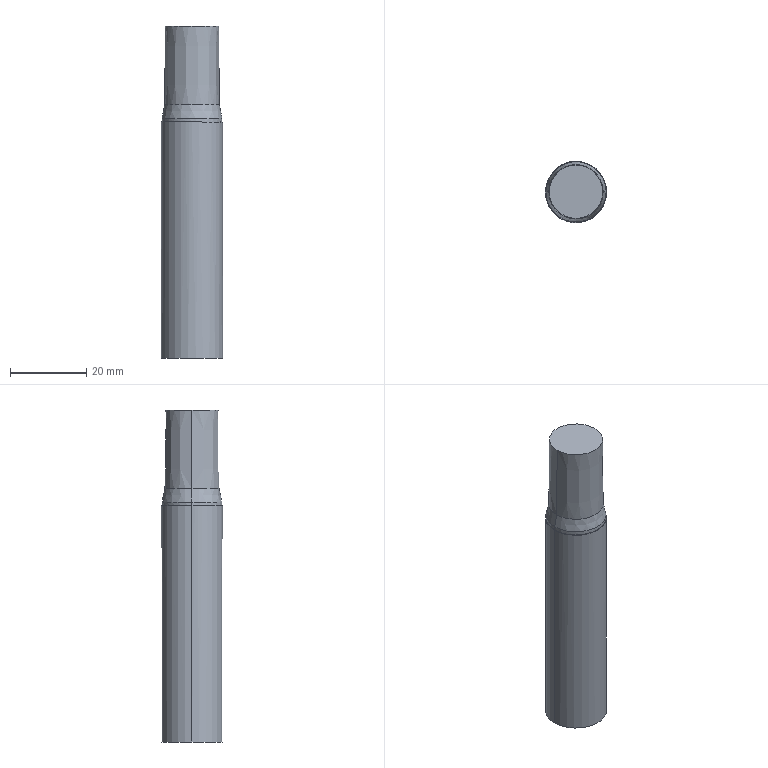Part | Creo | 1 solid | 12 faces | box 16 x 16 x 86.921 mm | volume 16469 mm3 | cylinder 4 | cone 4 | plane 3 | spline 1 | commonest cylinder face diameters 15.678 x2 16 x2
STEP:
#1=CARTESIAN_POINT('',(0.,0.,0.));
#2=DIRECTION('',(0.,0.,1.));
#3=DIRECTION('',(1.,0.,0.));
#4=AXIS2_PLACEMENT_3D('',#1,#2,#3);
#5=CARTESIAN_POINT('',(91.264,-22.481,-153.441));
#6=VERTEX_POINT('',#5);
#7=CARTESIAN_POINT('',(107.264,-22.481,-153.441));
#8=VERTEX_POINT('',#7);
#9=CARTESIAN_POINT('',(99.264,-22.481,-153.441));
#10=DIRECTION('',(0.,0.,-1.));
#11=DIRECTION('',(-1.,0.,0.));
#12=AXIS2_PLACEMENT_3D('',#9,#10,#11);
#13=CIRCLE('',#12,8.);
#14=EDGE_CURVE('',#6,#8,#13,.T.);
#15=ORIENTED_EDGE('',*,*,#14,.T.);
#16=CARTESIAN_POINT('',(107.264,-22.481,-91.656));
#17=VERTEX_POINT('',#16);
#18=CARTESIAN_POINT('',(107.264,-22.481,-91.656));
#19=DIRECTION('',(0.000000025,0.,-1.));
#20=VECTOR('',#19,61.786);
#21=LINE('',#18,#20);
#22=EDGE_CURVE('',#17,#8,#21,.T.);
#23=ORIENTED_EDGE('',*,*,#22,.F.);
#24=CARTESIAN_POINT('',(98.802,-14.494,-91.645));
#25=VERTEX_POINT('',#24);
#26=CARTESIAN_POINT('',(98.802,-14.494,-91.645));
#27=CARTESIAN_POINT('',(99.289,-14.466,-91.645));
#28=CARTESIAN_POINT('',(100.25,-14.498,-91.646));
#29=CARTESIAN_POINT('',(101.673,-14.806,-91.648));
#30=CARTESIAN_POINT('',(103.014,-15.365,-91.65));
#31=CARTESIAN_POINT('',(104.234,-16.156,-91.652));
#32=CARTESIAN_POINT('',(105.291,-17.154,-91.653));
#33=CARTESIAN_POINT('',(106.151,-18.326,-91.654));
#34=CARTESIAN_POINT('',(106.787,-19.632,-91.655));
#35=CARTESIAN_POINT('',(107.176,-21.036,-91.656));
#36=CARTESIAN_POINT('',(107.264,-21.993,-91.656));
#37=CARTESIAN_POINT('',(107.264,-22.481,-91.656));
#38=B_SPLINE_CURVE_WITH_KNOTS('',3,(#26,#27,#28,#29,#30,#31,#32,#33,#34,#35,#36,#37),.UNSPECIFIED.,.F.,.F.,(4,1,1,1,1,1,1,1,1,4),(0.,0.1111,0.2222,0.3333,0.4444,0.5556,0.6667,0.7778,0.8889,1.),.UNSPECIFIED.);
#39=EDGE_CURVE('',#25,#17,#38,.T.);
#40=ORIENTED_EDGE('',*,*,#39,.F.);
#41=CARTESIAN_POINT('',(96.482,-14.98,-91.641));
#42=VERTEX_POINT('',#41);
#43=CARTESIAN_POINT('',(96.73,-14.888,-91.642));
#44=CARTESIAN_POINT('',(97.235,-14.729,-91.643));
#45=CARTESIAN_POINT('',(98.012,-14.566,-91.644));
#46=CARTESIAN_POINT('',(98.538,-14.51,-91.644));
#47=CARTESIAN_POINT('',(98.802,-14.494,-91.645));
#48=B_SPLINE_CURVE_WITH_KNOTS('',3,(#41,#43,#44,#45,#46,#47),.UNSPECIFIED.,.F.,.F.,(4,1,1,4),(0.,0.3333,0.6667,1.),.UNSPECIFIED.);
#49=EDGE_CURVE('',#42,#25,#48,.T.);
#50=ORIENTED_EDGE('',*,*,#49,.F.);
#51=CARTESIAN_POINT('',(91.264,-22.482,-91.634));
#52=VERTEX_POINT('',#51);
#53=CARTESIAN_POINT('',(91.264,-22.482,-91.634));
#54=CARTESIAN_POINT('',(91.264,-22.258,-91.634));
#55=CARTESIAN_POINT('',(91.283,-21.784,-91.631));
#56=CARTESIAN_POINT('',(91.385,-21.015,-91.63));
#57=CARTESIAN_POINT('',(91.586,-20.173,-91.629));
#58=CARTESIAN_POINT('',(91.914,-19.269,-91.628));
#59=CARTESIAN_POINT('',(92.405,-18.31,-91.628));
#60=CARTESIAN_POINT('',(93.108,-17.318,-91.63));
#61=CARTESIAN_POINT('',(94.062,-16.35,-91.633));
#62=CARTESIAN_POINT('',(95.209,-15.538,-91.638));
#63=CARTESIAN_POINT('',(96.048,-15.141,-91.64));
#64=CARTESIAN_POINT('',(96.482,-14.98,-91.641));
#65=B_SPLINE_CURVE_WITH_KNOTS('',3,(#53,#54,#55,#56,#57,#58,#59,#60,#61,#62,#63,#64),.UNSPECIFIED.,.F.,.F.,(4,1,1,1,1,1,1,1,1,4),(0.,0.1111,0.2222,0.3333,0.4444,0.5556,0.6667,0.7778,0.8889,1.),.UNSPECIFIED.);
#66=EDGE_CURVE('',#52,#42,#65,.T.);
#67=ORIENTED_EDGE('',*,*,#66,.F.);
#68=CARTESIAN_POINT('',(91.264,-22.482,-91.634));
#69=DIRECTION('',(0.000000941,0.00001503,-1.));
#70=VECTOR('',#69,61.807);
#71=LINE('',#68,#70);
#72=EDGE_CURVE('',#52,#6,#71,.T.);
#73=ORIENTED_EDGE('',*,*,#72,.T.);
#74=EDGE_LOOP('',(#15,#23,#40,#50,#67,#73));
#75=FACE_OUTER_BOUND('',#74,.F.);
#76=CARTESIAN_POINT('',(99.264,-22.481,508.193));
#77=DIRECTION('',(0.,0.,-1.));
#78=DIRECTION('',(-1.,0.,0.));
#79=AXIS2_PLACEMENT_3D('',#76,#77,#78);
#80=CYLINDRICAL_SURFACE('',#79,8.);
#81=ADVANCED_FACE('',(#75),#80,.T.);
#82=ORIENTED_EDGE('',*,*,#14,.F.);
#83=CARTESIAN_POINT('',(99.264,-22.481,-153.441));
#84=DIRECTION('',(0.,0.,-1.));
#85=DIRECTION('',(1.,0.,0.));
#86=AXIS2_PLACEMENT_3D('',#83,#84,#85);
#87=CIRCLE('',#86,8.);
#88=EDGE_CURVE('',#8,#6,#87,.T.);
#89=ORIENTED_EDGE('',*,*,#88,.F.);
#90=EDGE_LOOP('',(#82,#89));
#91=FACE_OUTER_BOUND('',#90,.F.);
#92=CARTESIAN_POINT('',(5.725,319.968,-153.441));
#93=DIRECTION('',(0.,0.,-1.));
#94=DIRECTION('',(-1.,0.,0.));
#95=AXIS2_PLACEMENT_3D('',#92,#93,#94);
#96=PLANE('',#95);
#97=ADVANCED_FACE('',(#91),#96,.T.);
#98=ORIENTED_EDGE('',*,*,#88,.T.);
#99=ORIENTED_EDGE('',*,*,#72,.F.);
#100=CARTESIAN_POINT('',(96.482,-29.982,-91.641));
#101=VERTEX_POINT('',#100);
#102=CARTESIAN_POINT('',(96.046,-29.82,-91.64));
#103=CARTESIAN_POINT('',(95.205,-29.423,-91.638));
#104=CARTESIAN_POINT('',(94.055,-28.606,-91.633));
#105=CARTESIAN_POINT('',(93.102,-27.637,-91.63));
#106=CARTESIAN_POINT('',(92.402,-26.646,-91.628));
#107=CARTESIAN_POINT('',(91.912,-25.69,-91.628));
#108=CARTESIAN_POINT('',(91.586,-24.788,-91.629));
#109=CARTESIAN_POINT('',(91.385,-23.948,-91.63));
#110=CARTESIAN_POINT('',(91.283,-23.181,-91.631));
#111=CARTESIAN_POINT('',(91.264,-22.708,-91.634));
#112=CARTESIAN_POINT('',(91.264,-22.482,-91.634));
#113=B_SPLINE_CURVE_WITH_KNOTS('',3,(#100,#102,#103,#104,#105,#106,#107,#108,#109,#110,#111,#112),.UNSPECIFIED.,.F.,.F.,(4,1,1,1,1,1,1,1,1,4),(0.,0.1111,0.2222,0.3333,0.4444,0.5556,0.6667,0.7778,0.8889,1.),.UNSPECIFIED.);
#114=EDGE_CURVE('',#101,#52,#113,.T.);
#115=ORIENTED_EDGE('',*,*,#114,.F.);
#116=CARTESIAN_POINT('',(99.272,-30.481,-91.646));
#117=VERTEX_POINT('',#116);
#118=CARTESIAN_POINT('',(96.482,-29.982,-91.641));
#119=CARTESIAN_POINT('',(96.647,-30.043,-91.642));
#120=CARTESIAN_POINT('',(96.97,-30.15,-91.642));
#121=CARTESIAN_POINT('',(97.428,-30.272,-91.643));
#122=CARTESIAN_POINT('',(97.86,-30.361,-91.644));
#123=CARTESIAN_POINT('',(98.263,-30.421,-91.644));
#124=CARTESIAN_POINT('',(98.634,-30.459,-91.645));
#125=CARTESIAN_POINT('',(98.972,-30.478,-91.645));
#126=CARTESIAN_POINT('',(99.176,-30.481,-91.646));
#127=B_SPLINE_CURVE_WITH_KNOTS('',3,(#118,#119,#120,#121,#122,#123,#124,#125,#126,#116),.UNSPECIFIED.,.F.,.F.,(4,1,1,1,1,1,1,4),(0.,0.1429,0.2857,0.4286,0.5714,0.7143,0.8571,1.),.UNSPECIFIED.);
#128=EDGE_CURVE('',#101,#117,#127,.T.);
#129=ORIENTED_EDGE('',*,*,#128,.T.);
#130=CARTESIAN_POINT('',(106.717,-25.387,-91.659));
#131=VERTEX_POINT('',#130);
#132=CARTESIAN_POINT('',(99.272,-30.481,-91.646));
#133=CARTESIAN_POINT('',(99.437,-30.481,-91.646));
#134=CARTESIAN_POINT('',(99.781,-30.47,-91.647));
#135=CARTESIAN_POINT('',(100.332,-30.416,-91.649));
#136=CARTESIAN_POINT('',(100.93,-30.314,-91.651));
#137=CARTESIAN_POINT('',(101.576,-30.15,-91.653));
#138=CARTESIAN_POINT('',(102.274,-29.907,-91.655));
#139=CARTESIAN_POINT('',(103.018,-29.563,-91.658));
#140=CARTESIAN_POINT('',(103.8,-29.094,-91.66));
#141=CARTESIAN_POINT('',(104.602,-28.472,-91.662));
#142=CARTESIAN_POINT('',(105.392,-27.669,-91.663));
#143=CARTESIAN_POINT('',(106.129,-26.658,-91.667));
#144=CARTESIAN_POINT('',(106.542,-25.836,-91.66));
#145=CARTESIAN_POINT('',(106.717,-25.387,-91.659));
#146=B_SPLINE_CURVE_WITH_KNOTS('',3,(#132,#133,#134,#135,#136,#137,#138,#139,#140,#141,#142,#143,#144,#145),.UNSPECIFIED.,.F.,.F.,(4,1,1,1,1,1,1,1,1,1,1,4),(0.,0.09091,0.1818,0.2727,0.3636,0.4545,0.5455,0.6364,0.7273,0.8182,0.9091,1.),.UNSPECIFIED.);
#147=EDGE_CURVE('',#117,#131,#146,.T.);
#148=ORIENTED_EDGE('',*,*,#147,.T.);
#149=CARTESIAN_POINT('',(106.717,-25.387,-91.659));
#150=CARTESIAN_POINT('',(106.839,-25.074,-91.66));
#151=CARTESIAN_POINT('',(107.04,-24.443,-91.653));
#152=CARTESIAN_POINT('',(107.223,-23.471,-91.656));
#153=CARTESIAN_POINT('',(107.264,-22.813,-91.656));
#154=CARTESIAN_POINT('',(107.264,-22.481,-91.656));
#155=B_SPLINE_CURVE_WITH_KNOTS('',3,(#149,#150,#151,#152,#153,#154),.UNSPECIFIED.,.F.,.F.,(4,1,1,4),(0.,0.3333,0.6667,1.),.UNSPECIFIED.);
#156=EDGE_CURVE('',#131,#17,#155,.T.);
#157=ORIENTED_EDGE('',*,*,#156,.T.);
#158=ORIENTED_EDGE('',*,*,#22,.T.);
#159=EDGE_LOOP('',(#98,#99,#115,#129,#148,#157,#158));
#160=FACE_OUTER_BOUND('',#159,.F.);
#161=CARTESIAN_POINT('',(99.264,-22.481,508.193));
#162=DIRECTION('',(0.,0.,-1.));
#163=DIRECTION('',(-1.,0.,0.));
#164=AXIS2_PLACEMENT_3D('',#161,#162,#163);
#165=CYLINDRICAL_SURFACE('',#164,8.);
#166=ADVANCED_FACE('',(#160),#165,.T.);
#167=ORIENTED_EDGE('',*,*,#128,.F.);
#168=ORIENTED_EDGE('',*,*,#114,.T.);
#169=ORIENTED_EDGE('',*,*,#66,.T.);
#170=ORIENTED_EDGE('',*,*,#49,.T.);
#171=CARTESIAN_POINT('',(98.801,-14.656,-91.645));
#172=VERTEX_POINT('',#171);
#173=CARTESIAN_POINT('',(98.801,-14.637,-91.645));
#174=CARTESIAN_POINT('',(98.802,-14.599,-91.644));
#175=CARTESIAN_POINT('',(98.801,-14.54,-91.645));
#176=CARTESIAN_POINT('',(98.802,-14.509,-91.645));
#177=B_SPLINE_CURVE_WITH_KNOTS('',3,(#171,#173,#174,#175,#176,#24),.UNSPECIFIED.,.F.,.F.,(4,1,1,4),(0.,0.3333,0.6667,1.),.UNSPECIFIED.);
#178=EDGE_CURVE('',#172,#25,#177,.T.);
#179=ORIENTED_EDGE('',*,*,#178,.F.);
#180=CARTESIAN_POINT('',(91.425,-22.481,-91.63));
#181=VERTEX_POINT('',#180);
#182=CARTESIAN_POINT('',(91.425,-22.481,-91.63));
#183=CARTESIAN_POINT('',(91.425,-22.402,-91.63));
#184=CARTESIAN_POINT('',(91.427,-22.232,-91.63));
#185=CARTESIAN_POINT('',(91.441,-21.947,-91.63));
#186=CARTESIAN_POINT('',(91.469,-21.627,-91.63));
#187=CARTESIAN_POINT('',(91.516,-21.268,-91.629));
#188=CARTESIAN_POINT('',(91.589,-20.866,-91.629));
#189=CARTESIAN_POINT('',(91.695,-20.422,-91.629));
#190=CARTESIAN_POINT('',(91.844,-19.932,-91.628));
#191=CARTESIAN_POINT('',(92.051,-19.389,-91.628));
#192=CARTESIAN_POINT('',(92.335,-18.793,-91.628));
#193=CARTESIAN_POINT('',(92.708,-18.161,-91.629));
#194=CARTESIAN_POINT('',(93.158,-17.545,-91.63));
#195=CARTESIAN_POINT('',(93.666,-16.976,-91.631));
#196=CARTESIAN_POINT('',(94.223,-16.462,-91.633));
#197=CARTESIAN_POINT('',(94.833,-15.999,-91.636));
#198=CARTESIAN_POINT('',(95.447,-15.623,-91.638));
#199=CARTESIAN_POINT('',(96.026,-15.333,-91.64));
#200=CARTESIAN_POINT('',(96.553,-15.119,-91.641));
#201=CARTESIAN_POINT('',(97.026,-14.963,-91.643));
#202=CARTESIAN_POINT('',(97.457,-14.849,-91.643));
#203=CARTESIAN_POINT('',(97.85,-14.767,-91.644));
#204=CARTESIAN_POINT('',(98.204,-14.711,-91.645));
#205=CARTESIAN_POINT('',(98.521,-14.675,-91.646));
#206=CARTESIAN_POINT('',(98.712,-14.661,-91.645));
#207=CARTESIAN_POINT('',(98.801,-14.656,-91.645));
#208=B_SPLINE_CURVE_WITH_KNOTS('',3,(#182,#183,#184,#185,#186,#187,#188,#189,#190,#191,#192,#193,#194,#195,#196,#197,#198,#199,#200,#201,#202,#203,#204,#205,#206,#207),.UNSPECIFIED.,.F.,.F.,(4,1,1,1,1,1,1,1,1,1,1,1,1,1,1,1,1,1,1,1,1,1,1,4),(0.,0.04348,0.08696,0.1304,0.1739,0.2174,0.2609,0.3043,0.3478,0.3913,0.4348,0.4783,0.5217,0.5652,0.6087,0.6522,0.6957,0.7391,0.7826,0.8261,0.8696,0.913,0.9565,1.),.UNSPECIFIED.);
#209=EDGE_CURVE('',#181,#172,#208,.T.);
#210=ORIENTED_EDGE('',*,*,#209,.F.);
#211=CARTESIAN_POINT('',(106.544,-25.388,-91.66));
#212=VERTEX_POINT('',#211);
#213=CARTESIAN_POINT('',(106.544,-25.388,-91.66));
#214=CARTESIAN_POINT('',(106.45,-25.622,-91.66));
#215=CARTESIAN_POINT('',(106.242,-26.079,-91.667));
#216=CARTESIAN_POINT('',(105.867,-26.727,-91.664));
#217=CARTESIAN_POINT('',(105.433,-27.336,-91.664));
#218=CARTESIAN_POINT('',(104.941,-27.904,-91.663));
#219=CARTESIAN_POINT('',(104.388,-28.429,-91.662));
#220=CARTESIAN_POINT('',(103.798,-28.89,-91.66));
#221=CARTESIAN_POINT('',(103.201,-29.271,-91.658));
#222=CARTESIAN_POINT('',(102.631,-29.569,-91.657));
#223=CARTESIAN_POINT('',(102.114,-29.79,-91.655));
#224=CARTESIAN_POINT('',(101.644,-29.955,-91.654));
#225=CARTESIAN_POINT('',(101.214,-30.077,-91.652));
#226=CARTESIAN_POINT('',(100.825,-30.166,-91.651));
#227=CARTESIAN_POINT('',(100.476,-30.228,-91.65));
#228=CARTESIAN_POINT('',(100.159,-30.271,-91.649));
#229=CARTESIAN_POINT('',(99.866,-30.299,-91.648));
#230=CARTESIAN_POINT('',(99.587,-30.315,-91.648));
#231=CARTESIAN_POINT('',(99.317,-30.321,-91.647));
#232=CARTESIAN_POINT('',(99.049,-30.319,-91.646));
#233=CARTESIAN_POINT('',(98.778,-30.306,-91.646));
#234=CARTESIAN_POINT('',(98.497,-30.284,-91.645));
#235=CARTESIAN_POINT('',(98.197,-30.249,-91.645));
#236=CARTESIAN_POINT('',(97.871,-30.198,-91.644));
#237=CARTESIAN_POINT('',(97.508,-30.124,-91.644));
#238=CARTESIAN_POINT('',(97.106,-30.021,-91.643));
#239=CARTESIAN_POINT('',(96.662,-29.881,-91.642));
#240=CARTESIAN_POINT('',(96.176,-29.693,-91.64));
#241=CARTESIAN_POINT('',(95.644,-29.444,-91.639));
#242=CARTESIAN_POINT('',(95.066,-29.114,-91.637));
#243=CARTESIAN_POINT('',(94.472,-28.7,-91.634));
#244=CARTESIAN_POINT('',(93.899,-28.213,-91.632));
#245=CARTESIAN_POINT('',(93.37,-27.667,-91.63));
#246=CARTESIAN_POINT('',(92.9,-27.079,-91.629));
#247=CARTESIAN_POINT('',(92.5,-26.465,-91.628));
#248=CARTESIAN_POINT('',(92.184,-25.867,-91.628));
#249=CARTESIAN_POINT('',(91.95,-25.32,-91.628));
#250=CARTESIAN_POINT('',(91.777,-24.823,-91.629));
#251=CARTESIAN_POINT('',(91.652,-24.372,-91.629));
#252=CARTESIAN_POINT('',(91.563,-23.963,-91.629));
#253=CARTESIAN_POINT('',(91.501,-23.594,-91.63));
#254=CARTESIAN_POINT('',(91.462,-23.262,-91.63));
#255=CARTESIAN_POINT('',(91.438,-22.966,-91.63));
#256=CARTESIAN_POINT('',(91.427,-22.705,-91.63));
#257=CARTESIAN_POINT('',(91.425,-22.552,-91.63));
#258=CARTESIAN_POINT('',(91.425,-22.481,-91.63));
#259=B_SPLINE_CURVE_WITH_KNOTS('',3,(#213,#214,#215,#216,#217,#218,#219,#220,#221,#222,#223,#224,#225,#226,#227,#228,#229,#230,#231,#232,#233,#234,#235,#236,#237,#238,#239,#240,#241,#242,#243,#244,#245,#246,#247,#248,#249,#250,#251,#252,#253,#254,#255,#256,#257,#258),.UNSPECIFIED.,.F.,.F.,(4,1,1,1,1,1,1,1,1,1,1,1,1,1,1,1,1,1,1,1,1,1,1,1,1,1,1,1,1,1,1,1,1,1,1,1,1,1,1,1,1,1,1,4),(0.,0.02326,0.04651,0.06977,0.09302,0.1163,0.1395,0.1628,0.186,0.2093,0.2326,0.2558,0.2791,0.3023,0.3256,0.3488,0.3721,0.3953,0.4186,0.4419,0.4651,0.4884,0.5116,0.5349,0.5581,0.5814,0.6047,0.6279,0.6512,0.6744,0.6977,0.7209,0.7442,0.7674,0.7907,0.814,0.8372,0.8605,0.8837,0.907,0.9302,0.9535,0.9767,1.),.UNSPECIFIED.);
#260=EDGE_CURVE('',#212,#181,#259,.T.);
#261=ORIENTED_EDGE('',*,*,#260,.F.);
#262=CARTESIAN_POINT('',(106.7,-25.387,-91.659));
#263=CARTESIAN_POINT('',(106.664,-25.389,-91.654));
#264=CARTESIAN_POINT('',(106.603,-25.388,-91.653));
#265=CARTESIAN_POINT('',(106.564,-25.388,-91.66));
#266=B_SPLINE_CURVE_WITH_KNOTS('',3,(#130,#262,#263,#264,#265,#211),.UNSPECIFIED.,.F.,.F.,(4,1,1,4),(0.,0.3333,0.6667,1.),.UNSPECIFIED.);
#267=EDGE_CURVE('',#131,#212,#266,.T.);
#268=ORIENTED_EDGE('',*,*,#267,.F.);
#269=ORIENTED_EDGE('',*,*,#147,.F.);
#270=EDGE_LOOP('',(#167,#168,#169,#170,#179,#210,#261,#268,#269));
#271=FACE_OUTER_BOUND('',#270,.F.);
#272=CARTESIAN_POINT('',(91.252,-22.48,-91.636));
#273=CARTESIAN_POINT('',(91.208,-21.387,-91.631));
#274=CARTESIAN_POINT('',(91.579,-19.243,-91.627));
#275=CARTESIAN_POINT('',(93.345,-16.572,-91.629));
#276=CARTESIAN_POINT('',(95.851,-14.897,-91.641));
#277=CARTESIAN_POINT('',(97.776,-14.499,-91.643));
#278=CARTESIAN_POINT('',(98.675,-14.468,-91.644));
#279=CARTESIAN_POINT('',(91.21,-23.575,-91.631));
#280=CARTESIAN_POINT('',(91.36,-22.482,-91.628));
#281=CARTESIAN_POINT('',(92.071,-20.299,-91.626));
#282=CARTESIAN_POINT('',(94.197,-17.423,-91.631));
#283=CARTESIAN_POINT('',(96.896,-15.41,-91.644));
#284=CARTESIAN_POINT('',(98.864,-14.71,-91.646));
#285=CARTESIAN_POINT('',(99.769,-14.525,-91.648));
#286=CARTESIAN_POINT('',(91.585,-25.722,-91.627));
#287=CARTESIAN_POINT('',(92.075,-24.667,-91.626));
#288=CARTESIAN_POINT('',(93.377,-22.483,-91.628));
#289=CARTESIAN_POINT('',(96.096,-19.316,-91.637));
#290=CARTESIAN_POINT('',(99.066,-16.748,-91.65));
#291=CARTESIAN_POINT('',(101.049,-15.523,-91.654));
#292=CARTESIAN_POINT('',(101.933,-15.069,-91.655));
#293=CARTESIAN_POINT('',(93.358,-28.393,-91.629));
#294=CARTESIAN_POINT('',(94.208,-27.542,-91.631));
#295=CARTESIAN_POINT('',(96.102,-25.648,-91.637));
#296=CARTESIAN_POINT('',(99.274,-22.481,-91.648));
#297=CARTESIAN_POINT('',(102.246,-19.491,-91.661));
#298=CARTESIAN_POINT('',(103.988,-17.75,-91.663));
#299=CARTESIAN_POINT('',(104.721,-17.017,-91.664));
#300=CARTESIAN_POINT('',(96.023,-30.17,-91.642));
#301=CARTESIAN_POINT('',(97.077,-29.676,-91.645));
#302=CARTESIAN_POINT('',(99.26,-28.371,-91.651));
#303=CARTESIAN_POINT('',(102.434,-25.651,-91.661));
#304=CARTESIAN_POINT('',(104.984,-22.661,-91.669));
#305=CARTESIAN_POINT('',(106.212,-20.679,-91.668));
#306=CARTESIAN_POINT('',(106.666,-19.794,-91.666));
#307=CARTESIAN_POINT('',(98.162,-30.533,-91.644));
#308=CARTESIAN_POINT('',(99.255,-30.378,-91.647));
#309=CARTESIAN_POINT('',(101.438,-29.663,-91.654));
#310=CARTESIAN_POINT('',(104.324,-27.534,-91.664));
#311=CARTESIAN_POINT('',(106.321,-24.817,-91.667));
#312=CARTESIAN_POINT('',(107.027,-22.851,-91.664));
#313=CARTESIAN_POINT('',(107.214,-21.946,-91.662));
#314=CARTESIAN_POINT('',(99.248,-30.494,-91.645));
#315=CARTESIAN_POINT('',(100.341,-30.53,-91.648));
#316=CARTESIAN_POINT('',(102.486,-30.153,-91.656));
#317=CARTESIAN_POINT('',(105.171,-28.379,-91.664));
#318=CARTESIAN_POINT('',(106.834,-25.854,-91.665));
#319=CARTESIAN_POINT('',(107.241,-23.929,-91.661));
#320=CARTESIAN_POINT('',(107.276,-23.03,-91.657));
#321=B_SPLINE_SURFACE_WITH_KNOTS('',3,3,((#272,#273,#274,#275,#276,#277,#278),(#279,#280,#281,#282,#283,#284,#285),(#286,#287,#288,#289,#290,#291,#292),(#293,#294,#295,#296,#297,#298,#299),(#300,#301,#302,#303,#304,#305,#306),(#307,#308,#309,#310,#311,#312,#313),(#314,#315,#316,#317,#318,#319,#320)),.UNSPECIFIED.,.F.,.F.,.F.,(4,1,1,1,4),(4,1,1,1,4),(-0.01101,0.25,0.5,0.75,1.009),(-0.01051,0.25,0.5,0.75,0.9646),.UNSPECIFIED.);
#322=ADVANCED_FACE('',(#271),#321,.T.);
#323=ORIENTED_EDGE('',*,*,#39,.T.);
#324=ORIENTED_EDGE('',*,*,#156,.F.);
#325=ORIENTED_EDGE('',*,*,#267,.T.);
#326=CARTESIAN_POINT('',(107.103,-22.491,-91.656));
#327=VERTEX_POINT('',#326);
#328=CARTESIAN_POINT('',(107.103,-22.491,-91.656));
#329=CARTESIAN_POINT('',(107.102,-22.822,-91.656));
#330=CARTESIAN_POINT('',(107.06,-23.479,-91.656));
#331=CARTESIAN_POINT('',(106.872,-24.455,-91.653));
#332=CARTESIAN_POINT('',(106.667,-25.08,-91.66));
#333=CARTESIAN_POINT('',(106.544,-25.388,-91.66));
#334=B_SPLINE_CURVE_WITH_KNOTS('',3,(#328,#329,#330,#331,#332,#333),.UNSPECIFIED.,.F.,.F.,(4,1,1,4),(0.,0.3333,0.6667,1.),.UNSPECIFIED.);
#335=EDGE_CURVE('',#327,#212,#334,.T.);
#336=ORIENTED_EDGE('',*,*,#335,.F.);
#337=CARTESIAN_POINT('',(107.103,-22.481,-91.656));
#338=VERTEX_POINT('',#337);
#339=CARTESIAN_POINT('',(107.103,-22.488,-91.656));
#340=CARTESIAN_POINT('',(107.103,-22.484,-91.656));
#341=B_SPLINE_CURVE_WITH_KNOTS('',3,(#326,#339,#340,#337),.UNSPECIFIED.,.F.,.F.,(4,4),(0.,1.),.UNSPECIFIED.);
#342=EDGE_CURVE('',#327,#338,#341,.T.);
#343=ORIENTED_EDGE('',*,*,#342,.T.);
#344=CARTESIAN_POINT('',(107.103,-22.481,-91.656));
#345=CARTESIAN_POINT('',(107.103,-22.003,-91.656));
#346=CARTESIAN_POINT('',(107.017,-21.064,-91.655));
#347=CARTESIAN_POINT('',(106.634,-19.687,-91.655));
#348=CARTESIAN_POINT('',(106.011,-18.406,-91.654));
#349=CARTESIAN_POINT('',(105.167,-17.258,-91.653));
#350=CARTESIAN_POINT('',(104.129,-16.28,-91.652));
#351=CARTESIAN_POINT('',(102.933,-15.505,-91.65));
#352=CARTESIAN_POINT('',(101.617,-14.958,-91.648));
#353=CARTESIAN_POINT('',(100.221,-14.658,-91.646));
#354=CARTESIAN_POINT('',(99.278,-14.627,-91.646));
#355=CARTESIAN_POINT('',(98.801,-14.656,-91.645));
#356=B_SPLINE_CURVE_WITH_KNOTS('',3,(#344,#345,#346,#347,#348,#349,#350,#351,#352,#353,#354,#355),.UNSPECIFIED.,.F.,.F.,(4,1,1,1,1,1,1,1,1,4),(0.,0.1111,0.2222,0.3333,0.4444,0.5556,0.6667,0.7778,0.8889,1.),.UNSPECIFIED.);
#357=EDGE_CURVE('',#338,#172,#356,.T.);
#358=ORIENTED_EDGE('',*,*,#357,.T.);
#359=ORIENTED_EDGE('',*,*,#178,.T.);
#360=EDGE_LOOP('',(#323,#324,#325,#336,#343,#358,#359));
#361=FACE_OUTER_BOUND('',#360,.F.);
#362=CARTESIAN_POINT('',(248.993,54.022,-91.842));
#363=DIRECTION('',(-0.001312,0.000001665,-1.));
#364=DIRECTION('',(-1.,0.,0.001312));
#365=AXIS2_PLACEMENT_3D('',#362,#363,#364);
#366=PLANE('',#365);
#367=ADVANCED_FACE('',(#361),#366,.F.);
#368=CARTESIAN_POINT('',(91.423,-22.481,-90.64));
#369=VERTEX_POINT('',#368);
#370=CARTESIAN_POINT('',(107.103,-22.481,-90.64));
#371=VERTEX_POINT('',#370);
#372=CARTESIAN_POINT('',(99.263,-22.481,-90.64));
#373=DIRECTION('',(0.00002709,0.,1.));
#374=DIRECTION('',(-1.,0.,0.00002709));
#375=AXIS2_PLACEMENT_3D('',#372,#373,#374);
#376=CIRCLE('',#375,7.841);
#377=EDGE_CURVE('',#369,#371,#376,.T.);
#378=ORIENTED_EDGE('',*,*,#377,.T.);
#379=CARTESIAN_POINT('',(107.103,-22.481,-91.656));
#380=DIRECTION('',(0.0003875,0.,1.));
#381=VECTOR('',#380,1.015);
#382=LINE('',#379,#381);
#383=EDGE_CURVE('',#338,#371,#382,.T.);
#384=ORIENTED_EDGE('',*,*,#383,.F.);
#385=ORIENTED_EDGE('',*,*,#342,.F.);
#386=ORIENTED_EDGE('',*,*,#335,.T.);
#387=ORIENTED_EDGE('',*,*,#260,.T.);
#388=CARTESIAN_POINT('',(91.425,-22.481,-91.63));
#389=DIRECTION('',(-0.001845,0.000000928,1.));
#390=VECTOR('',#389,0.9902);
#391=LINE('',#388,#390);
#392=EDGE_CURVE('',#181,#369,#391,.T.);
#393=ORIENTED_EDGE('',*,*,#392,.T.);
#394=EDGE_LOOP('',(#378,#384,#385,#386,#387,#393));
#395=FACE_OUTER_BOUND('',#394,.F.);
#396=CARTESIAN_POINT('',(99.264,-22.481,-91.645));
#397=DIRECTION('',(0.,0.,1.));
#398=DIRECTION('',(1.,0.,0.));
#399=AXIS2_PLACEMENT_3D('',#396,#397,#398);
#400=CYLINDRICAL_SURFACE('',#399,7.839);
#401=ADVANCED_FACE('',(#395),#400,.T.);
#402=CARTESIAN_POINT('',(92.127,-22.481,-87.122));
#403=VERTEX_POINT('',#402);
#404=CARTESIAN_POINT('',(106.4,-22.481,-87.123));
#405=VERTEX_POINT('',#404);
#406=CARTESIAN_POINT('',(99.264,-22.481,-87.123));
#407=DIRECTION('',(0.,0.,1.));
#408=DIRECTION('',(-1.,0.,0.));
#409=AXIS2_PLACEMENT_3D('',#406,#407,#408);
#410=CIRCLE('',#409,7.136);
#411=EDGE_CURVE('',#403,#405,#410,.T.);
#412=ORIENTED_EDGE('',*,*,#411,.T.);
#413=CARTESIAN_POINT('',(106.4,-22.481,-87.123));
#414=DIRECTION('',(0.1961,0.,-0.9806));
#415=VECTOR('',#414,3.587);
#416=LINE('',#413,#415);
#417=EDGE_CURVE('',#405,#371,#416,.T.);
#418=ORIENTED_EDGE('',*,*,#417,.T.);
#419=ORIENTED_EDGE('',*,*,#377,.F.);
#420=CARTESIAN_POINT('',(92.127,-22.481,-87.122));
#421=DIRECTION('',(-0.1962,0.,-0.9806));
#422=VECTOR('',#421,3.587);
#423=LINE('',#420,#422);
#424=EDGE_CURVE('',#403,#369,#423,.T.);
#425=ORIENTED_EDGE('',*,*,#424,.F.);
#426=EDGE_LOOP('',(#412,#418,#419,#425));
#427=FACE_OUTER_BOUND('',#426,.F.);
#428=CARTESIAN_POINT('',(99.263,-22.481,-88.881));
#429=DIRECTION('',(-0.00002709,0.,-1.));
#430=DIRECTION('',(1.,0.,-0.00002709));
#431=AXIS2_PLACEMENT_3D('',#428,#429,#430);
#432=CONICAL_SURFACE('',#431,7.489,11.313);
#433=ADVANCED_FACE('',(#427),#432,.T.);
#434=ORIENTED_EDGE('',*,*,#411,.F.);
#435=CARTESIAN_POINT('',(92.272,-22.481,-66.52));
#436=VERTEX_POINT('',#435);
#437=CARTESIAN_POINT('',(92.272,-22.481,-66.52));
#438=DIRECTION('',(-0.007046,0.,-1.));
#439=VECTOR('',#438,20.603);
#440=LINE('',#437,#439);
#441=EDGE_CURVE('',#436,#403,#440,.T.);
#442=ORIENTED_EDGE('',*,*,#441,.F.);
#443=CARTESIAN_POINT('',(106.255,-22.481,-66.52));
#444=VERTEX_POINT('',#443);
#445=CARTESIAN_POINT('',(99.264,-22.481,-66.52));
#446=DIRECTION('',(0.,0.,1.));
#447=DIRECTION('',(-1.,0.,0.));
#448=AXIS2_PLACEMENT_3D('',#445,#446,#447);
#449=CIRCLE('',#448,6.992);
#450=EDGE_CURVE('',#436,#444,#449,.T.);
#451=ORIENTED_EDGE('',*,*,#450,.T.);
#452=CARTESIAN_POINT('',(106.255,-22.481,-66.52));
#453=DIRECTION('',(0.006999,0.,-1.));
#454=VECTOR('',#453,20.603);
#455=LINE('',#452,#454);
#456=EDGE_CURVE('',#444,#405,#455,.T.);
#457=ORIENTED_EDGE('',*,*,#456,.T.);
#458=EDGE_LOOP('',(#434,#442,#451,#457));
#459=FACE_OUTER_BOUND('',#458,.F.);
#460=CARTESIAN_POINT('',(99.264,-22.481,-76.821));
#461=DIRECTION('',(0.,0.,-1.));
#462=DIRECTION('',(1.,0.,0.));
#463=AXIS2_PLACEMENT_3D('',#460,#461,#462);
#464=CONICAL_SURFACE('',#463,7.064,0.4);
#465=ADVANCED_FACE('',(#459),#464,.T.);
#466=CARTESIAN_POINT('',(99.264,-22.481,-87.123));
#467=DIRECTION('',(0.,0.,1.));
#468=DIRECTION('',(1.,0.,0.));
#469=AXIS2_PLACEMENT_3D('',#466,#467,#468);
#470=CIRCLE('',#469,7.136);
#471=EDGE_CURVE('',#405,#403,#470,.T.);
#472=ORIENTED_EDGE('',*,*,#471,.F.);
#473=ORIENTED_EDGE('',*,*,#456,.F.);
#474=CARTESIAN_POINT('',(99.264,-22.481,-66.52));
#475=DIRECTION('',(0.,0.,1.));
#476=DIRECTION('',(1.,0.,0.));
#477=AXIS2_PLACEMENT_3D('',#474,#475,#476);
#478=CIRCLE('',#477,6.992);
#479=EDGE_CURVE('',#444,#436,#478,.T.);
#480=ORIENTED_EDGE('',*,*,#479,.T.);
#481=ORIENTED_EDGE('',*,*,#441,.T.);
#482=EDGE_LOOP('',(#472,#473,#480,#481));
#483=FACE_OUTER_BOUND('',#482,.F.);
#484=CARTESIAN_POINT('',(99.264,-22.481,-76.821));
#485=DIRECTION('',(0.,0.,-1.));
#486=DIRECTION('',(1.,0.,0.));
#487=AXIS2_PLACEMENT_3D('',#484,#485,#486);
#488=CONICAL_SURFACE('',#487,7.064,0.4);
#489=ADVANCED_FACE('',(#483),#488,.T.);
#490=ORIENTED_EDGE('',*,*,#471,.T.);
#491=ORIENTED_EDGE('',*,*,#424,.T.);
#492=CARTESIAN_POINT('',(99.263,-22.481,-90.64));
#493=DIRECTION('',(0.00002709,0.,1.));
#494=DIRECTION('',(1.,0.,-0.00002709));
#495=AXIS2_PLACEMENT_3D('',#492,#493,#494);
#496=CIRCLE('',#495,7.841);
#497=EDGE_CURVE('',#371,#369,#496,.T.);
#498=ORIENTED_EDGE('',*,*,#497,.F.);
#499=ORIENTED_EDGE('',*,*,#417,.F.);
#500=EDGE_LOOP('',(#490,#491,#498,#499));
#501=FACE_OUTER_BOUND('',#500,.F.);
#502=CARTESIAN_POINT('',(99.263,-22.481,-88.881));
#503=DIRECTION('',(-0.00002709,0.,-1.));
#504=DIRECTION('',(1.,0.,-0.00002709));
#505=AXIS2_PLACEMENT_3D('',#502,#503,#504);
#506=CONICAL_SURFACE('',#505,7.489,11.313);
#507=ADVANCED_FACE('',(#501),#506,.T.);
#508=ORIENTED_EDGE('',*,*,#497,.T.);
#509=ORIENTED_EDGE('',*,*,#392,.F.);
#510=ORIENTED_EDGE('',*,*,#209,.T.);
#511=ORIENTED_EDGE('',*,*,#357,.F.);
#512=ORIENTED_EDGE('',*,*,#383,.T.);
#513=EDGE_LOOP('',(#508,#509,#510,#511,#512));
#514=FACE_OUTER_BOUND('',#513,.F.);
#515=CARTESIAN_POINT('',(99.264,-22.481,-91.645));
#516=DIRECTION('',(0.,0.,1.));
#517=DIRECTION('',(1.,0.,0.));
#518=AXIS2_PLACEMENT_3D('',#515,#516,#517);
#519=CYLINDRICAL_SURFACE('',#518,7.839);
#520=ADVANCED_FACE('',(#514),#519,.T.);
#521=ORIENTED_EDGE('',*,*,#479,.F.);
#522=ORIENTED_EDGE('',*,*,#450,.F.);
#523=EDGE_LOOP('',(#521,#522));
#524=FACE_OUTER_BOUND('',#523,.F.);
#525=CARTESIAN_POINT('',(99.264,-22.481,-66.52));
#526=DIRECTION('',(0.,0.,1.));
#527=DIRECTION('',(1.,0.,0.));
#528=AXIS2_PLACEMENT_3D('',#525,#526,#527);
#529=PLANE('',#528);
#530=ADVANCED_FACE('',(#524),#529,.T.);
#531=CLOSED_SHELL('',(#81,#97,#166,#322,#367,#401,#433,#465,#489,#507,#520,#530));
#532=MANIFOLD_SOLID_BREP('',#531);
#533=(LENGTH_UNIT()NAMED_UNIT(*)SI_UNIT(.MILLI.,.METRE.));
#534=UNCERTAINTY_MEASURE_WITH_UNIT(LENGTH_MEASURE(0.00899),#533,'','');
#535=(NAMED_UNIT(*)PLANE_ANGLE_UNIT()SI_UNIT($,.RADIAN.));
#536=PLANE_ANGLE_MEASURE_WITH_UNIT(PLANE_ANGLE_MEASURE(0.01745),#535);
#537=(CONVERSION_BASED_UNIT('DEGREE',#536)NAMED_UNIT(*)PLANE_ANGLE_UNIT());
#538=(NAMED_UNIT(*)SI_UNIT($,.STERADIAN.)SOLID_ANGLE_UNIT());
#539=(GEOMETRIC_REPRESENTATION_CONTEXT(3)GLOBAL_UNCERTAINTY_ASSIGNED_CONTEXT((#534))GLOBAL_UNIT_ASSIGNED_CONTEXT((#533,#537,#538))REPRESENTATION_CONTEXT('',''));
#540=ADVANCED_BREP_SHAPE_REPRESENTATION('',(#4,#532),#539);